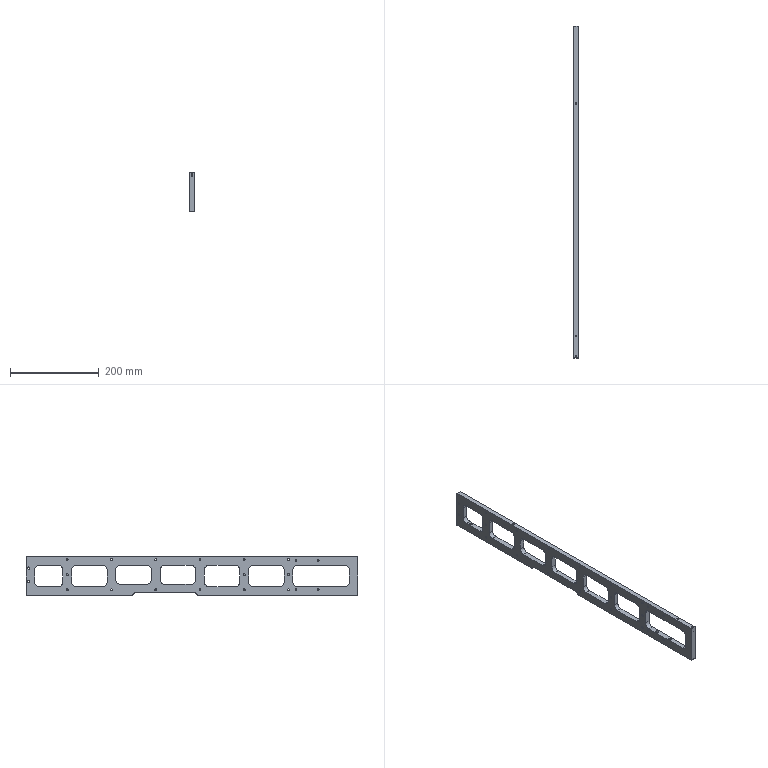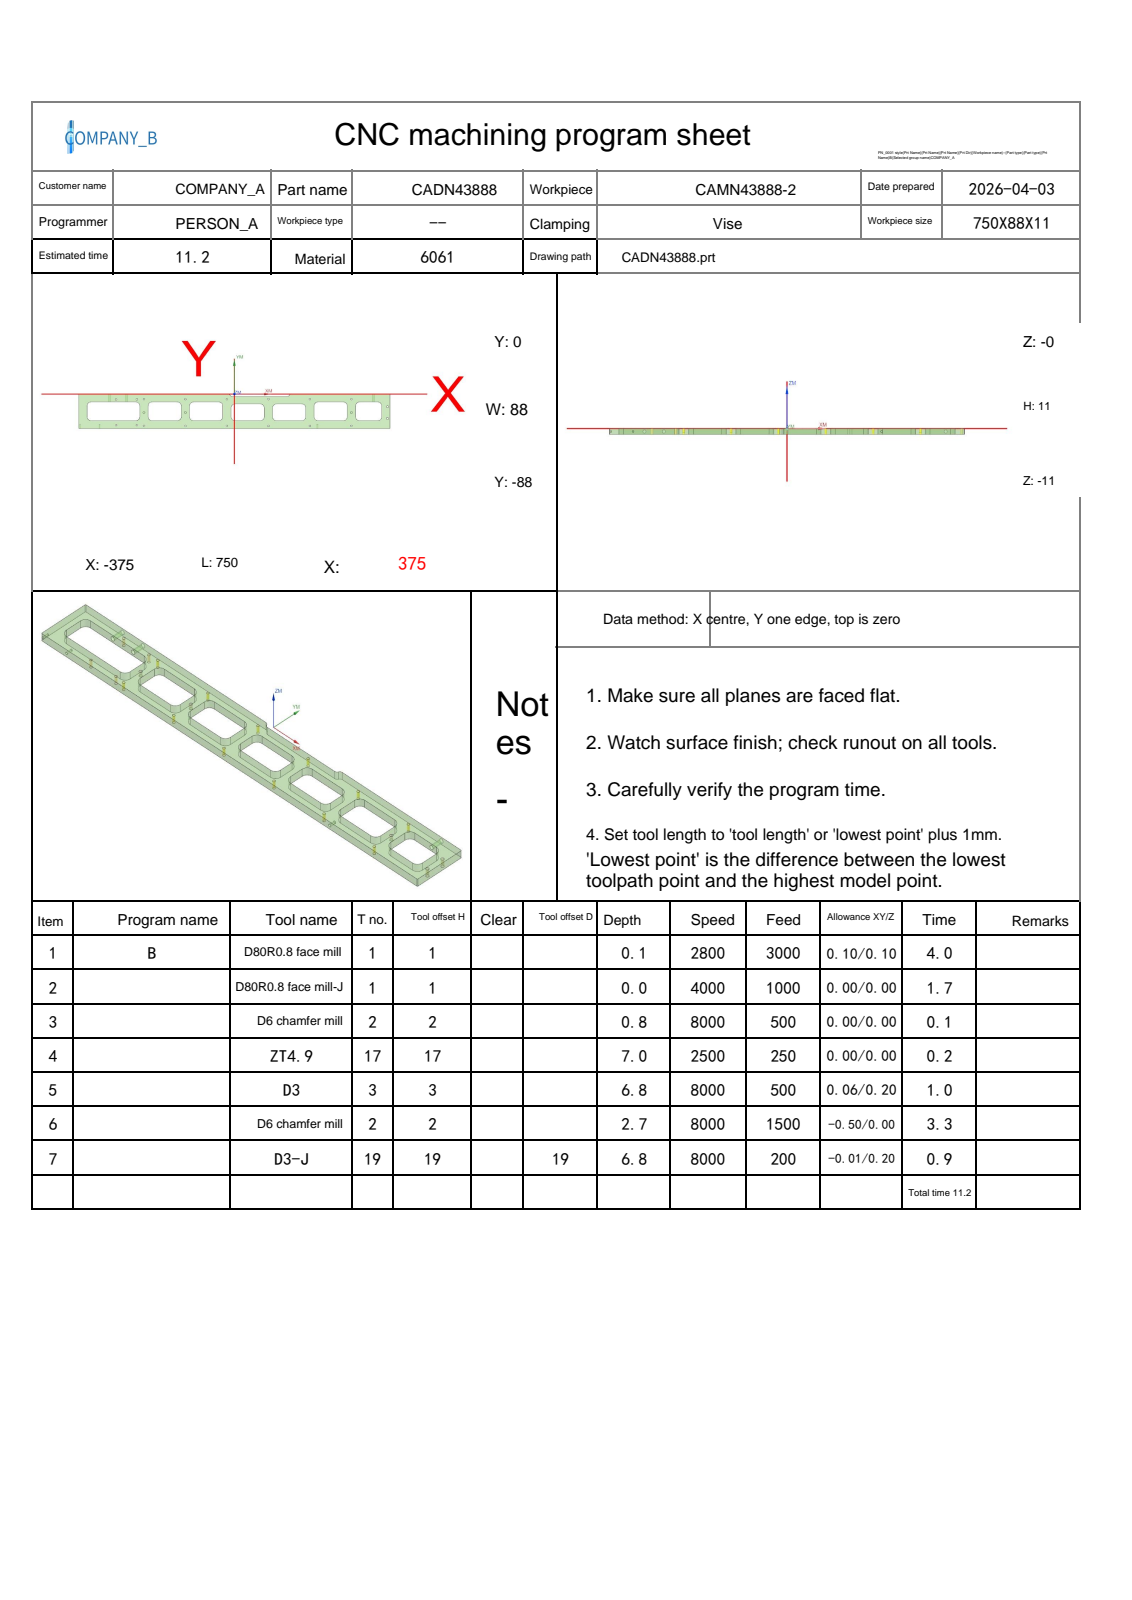NC program | NX | posted by the shop | part box 11 x 750 x 88 mm
Whole program:
%
O0001
(Machine time: 12.66 MIN)
(===Total Tool:5===)
(T1=D80R0.8 face mill D=80.  R=0.8  D-  H01 Z=-0.   )
(T2=D6 chamfer mill   D=6.   R=0.   D-  H02 Z=-2.7  )
(T17=ZT4.9  D=4.9  DR_a=120 D-  H17 Z=-7.   )
(T3=D3      D=3.   R=0.   D-  H03 Z=-6.8  )
(T19=D3-J   D=3.   R=0.   D19 H19 Z=-6.8  )
G80 G90 G17 G49 G40
G91 G28 Z0
M01
N1 T01 M06
(D80R0.8 face mill  D=80. R=0.8 H=01 ce=0.10 di=0.10)
G00 G90 G54 X-427.097 Y-24.494 M03 S2800
G43 H01 Z20.
M08
Z5.014
G01 Z3.014 F3000.
X-415.097 Y-24.361
X407.817 Y-15.229
X407.897
G02 X415.097 Y-22.429 I0.0 J-7.2
G01 Y-48.367
G02 X407.186 Y-56.366 I-8. J0.0
G01 X-415.097 Y-65.491
X-427.097 Y-65.624
Z5.014
G00 Y-24.494
Z4.529
G01 Z2.529
X-415.097 Y-24.361
X407.817 Y-15.229
X407.897
G02 X415.097 Y-22.429 I0.0 J-7.2
G01 Y-48.367
G02 X407.186 Y-56.366 I-8. J0.0
G01 X-415.097 Y-65.491
X-427.097 Y-65.624
Z4.529
G00 Y-24.494
Z4.043
G01 Z2.043
X-415.097 Y-24.361
X407.817 Y-15.229
X407.897
G02 X415.097 Y-22.429 I0.0 J-7.2
G01 Y-48.367
G02 X407.186 Y-56.366 I-8. J0.0
G01 X-415.097 Y-65.491
X-427.097 Y-65.624
Z4.043
G00 Y-24.494
Z3.557
G01 Z1.557
X-415.097 Y-24.361
X407.817 Y-15.229
X407.897
G02 X415.097 Y-22.429 I0.0 J-7.2
G01 Y-48.367
G02 X407.186 Y-56.366 I-8. J0.0
G01 X-415.097 Y-65.491
X-427.097 Y-65.624
Z3.557
G00 Y-24.494
Z3.071
G01 Z1.071
X-415.097 Y-24.361
X407.817 Y-15.229
X407.897
G02 X415.097 Y-22.429 I0.0 J-7.2
G01 Y-48.367
G02 X407.186 Y-56.366 I-8. J0.0
G01 X-415.097 Y-65.491
X-427.097 Y-65.624
Z3.071
G00 Y-24.494
Z2.586
G01 Z.586
X-415.097 Y-24.361
X407.817 Y-15.229
X407.897
G02 X415.097 Y-22.429 I0.0 J-7.2
G01 Y-48.367
G02 X407.186 Y-56.366 I-8. J0.0
G01 X-415.097 Y-65.491
X-427.097 Y-65.624
Z2.586
G00 Y-24.494
Z2.1
G01 Z.1
X-415.097 Y-24.361
X407.817 Y-15.229
X407.897
G02 X415.097 Y-22.429 I0.0 J-7.2
G01 Y-48.367
G02 X407.186 Y-56.366 I-8. J0.0
G01 X-415.097 Y-65.491
X-427.097 Y-65.624
Z2.1
G00 Z20.
G91 G28 Z0.0
M05
M09
G91 G28 Z0.0
M01
N2 T01 M06
(D80R0.8 face mill-J  D=80. R=0.8 H=01 ce=0.00 di=0.00)
G00 G90 G54 X-426.999 Y-24.589 M03 S4000
G43 H01 Z20.
M08
Z2.
G01 Z0.0 F1000.
X-414.999 Y-24.456
X407.719 Y-15.352
X407.799
G02 X414.999 Y-22.552 I0.0 J-7.2
G01 Y-48.271
G02 X407.088 Y-56.271 I-8. J0.0
G01 X-414.999 Y-65.368
X-426.999 Y-65.501
Z2.
G00 Z20.
G91 G28 Z0.0
M05
M09
G91 G28 Z0.0
M01
N3 T02 M06
(D6 chamfer mill  D=6. R=0. H=02 ce=0.00 di=0.00)
G00 G90 G54 X282. Y-47. M03 S8000
G43 H02 Z20.
M08
G98 G81 X282. Y-47. Z-.8 R1. F500.
X-118.
X-218.
G80
G00 Z20.
G91 G28 Z0.0
M05
M09
G91 G28 Z0.0
M01
N4 T17 M06
(ZT4.9 D=4.9 DR_a=120 H=17)
G00 G90 G54 X282. Y-47. M03 S2500
G43 H17 Z20.
M08
G98 G83 X282. Y-47. Z-7. R1. F250. Q2.
X-118.
X-218.
G80
G00 Z20.
G91 G28 Z0.0
M05
M09
G91 G28 Z0.0
M01
N5 T03 M06
(D3  D=3. R=0. H=03 ce=0.06 di=0.20)
G00 G90 G54 X282. Y-47. M03 S8000
G43 H03 Z20.
M08
Z.5
G03 X282.475 Y-47.475 I.475 J0.0 F500.
X282.95 Y-47. I0.0 J.475
X282.95 Y-47. Z.2 I-.95 J0.0
X282.95 Y-47. Z-.1 I-.95 J0.0
X282.95 Y-47. Z-.4 I-.95 J0.0
X282.95 Y-47. Z-.7 I-.95 J0.0
X282.95 Y-47. Z-1. I-.95 J0.0
X282.95 Y-47. Z-1.3 I-.95 J0.0
X282.95 Y-47. Z-1.6 I-.95 J0.0
X282.95 Y-47. Z-1.9 I-.95 J0.0
X282.95 Y-47. Z-2.2 I-.95 J0.0
X282.95 Y-47. Z-2.5 I-.95 J0.0
X282.95 Y-47. Z-2.8 I-.95 J0.0
X282.95 Y-47. Z-3.1 I-.95 J0.0
X282.95 Y-47. Z-3.4 I-.95 J0.0
X282.95 Y-47. Z-3.7 I-.95 J0.0
X282.95 Y-47. Z-4. I-.95 J0.0
X282.95 Y-47. Z-4.3 I-.95 J0.0
X282.95 Y-47. Z-4.6 I-.95 J0.0
X282.95 Y-47. Z-4.9 I-.95 J0.0
X282.95 Y-47. Z-5.2 I-.95 J0.0
X282.95 Y-47. Z-5.5 I-.95 J0.0
X282.95 Y-47. Z-5.8 I-.95 J0.0
X282.95 Y-47. Z-6.1 I-.95 J0.0
X282.95 Y-47. Z-6.4 I-.95 J0.0
X282.95 Y-47. Z-6.7 I-.95 J0.0
X281.525 Y-46.177 Z-6.8 I-.95 J0.0
X281.05 Y-47. I.475 J-.823
X282. Y-47.95 I.95 J0.0
X282.95 Y-47. I0.0 J.95
X282. Y-46.05 I-.95 J0.0
X281.525 Y-46.177 I0.0 J-.95
X281.288 Y-46.589 I.238 J-.411
X281.763 Y-47.064 I.475 J0.0
X282. Y-47. I0.0 J.475
G00 Z20.
X-118.
Z.5
G03 X-117.525 Y-47.475 I.475 J0.0
X-117.05 Y-47. I0.0 J.475
X-117.05 Y-47. Z.2 I-.95 J0.0
X-117.05 Y-47. Z-.1 I-.95 J0.0
X-117.05 Y-47. Z-.4 I-.95 J0.0
X-117.05 Y-47. Z-.7 I-.95 J0.0
X-117.05 Y-47. Z-1. I-.95 J0.0
X-117.05 Y-47. Z-1.3 I-.95 J0.0
X-117.05 Y-47. Z-1.6 I-.95 J0.0
X-117.05 Y-47. Z-1.9 I-.95 J0.0
X-117.05 Y-47. Z-2.2 I-.95 J0.0
X-117.05 Y-47. Z-2.5 I-.95 J0.0
X-117.05 Y-47. Z-2.8 I-.95 J0.0
X-117.05 Y-47. Z-3.1 I-.95 J0.0
X-117.05 Y-47. Z-3.4 I-.95 J0.0
X-117.05 Y-47. Z-3.7 I-.95 J0.0
X-117.05 Y-47. Z-4. I-.95 J0.0
X-117.05 Y-47. Z-4.3 I-.95 J0.0
X-117.05 Y-47. Z-4.6 I-.95 J0.0
X-117.05 Y-47. Z-4.9 I-.95 J0.0
X-117.05 Y-47. Z-5.2 I-.95 J0.0
X-117.05 Y-47. Z-5.5 I-.95 J0.0
X-117.05 Y-47. Z-5.8 I-.95 J0.0
X-117.05 Y-47. Z-6.1 I-.95 J0.0
X-117.05 Y-47. Z-6.4 I-.95 J0.0
X-117.05 Y-47. Z-6.7 I-.95 J0.0
X-118.475 Y-46.177 Z-6.8 I-.95 J0.0
X-118.95 Y-47. I.475 J-.823
X-118. Y-47.95 I.95 J0.0
X-117.05 Y-47. I0.0 J.95
X-118. Y-46.05 I-.95 J0.0
X-118.475 Y-46.177 I0.0 J-.95
X-118.712 Y-46.589 I.238 J-.411
X-118.237 Y-47.064 I.475 J0.0
X-118. Y-47. I0.0 J.475
G00 Z20.
X-218.
Z.5
G03 X-217.525 Y-47.475 I.475 J0.0
X-217.05 Y-47. I0.0 J.475
X-217.05 Y-47. Z.2 I-.95 J0.0
X-217.05 Y-47. Z-.1 I-.95 J0.0
X-217.05 Y-47. Z-.4 I-.95 J0.0
X-217.05 Y-47. Z-.7 I-.95 J0.0
X-217.05 Y-47. Z-1. I-.95 J0.0
X-217.05 Y-47. Z-1.3 I-.95 J0.0
X-217.05 Y-47. Z-1.6 I-.95 J0.0
X-217.05 Y-47. Z-1.9 I-.95 J0.0
X-217.05 Y-47. Z-2.2 I-.95 J0.0
X-217.05 Y-47. Z-2.5 I-.95 J0.0
X-217.05 Y-47. Z-2.8 I-.95 J0.0
X-217.05 Y-47. Z-3.1 I-.95 J0.0
X-217.05 Y-47. Z-3.4 I-.95 J0.0
X-217.05 Y-47. Z-3.7 I-.95 J0.0
X-217.05 Y-47. Z-4. I-.95 J0.0
X-217.05 Y-47. Z-4.3 I-.95 J0.0
X-217.05 Y-47. Z-4.6 I-.95 J0.0
X-217.05 Y-47. Z-4.9 I-.95 J0.0
X-217.05 Y-47. Z-5.2 I-.95 J0.0
X-217.05 Y-47. Z-5.5 I-.95 J0.0
X-217.05 Y-47. Z-5.8 I-.95 J0.0
X-217.05 Y-47. Z-6.1 I-.95 J0.0
X-217.05 Y-47. Z-6.4 I-.95 J0.0
X-217.05 Y-47. Z-6.7 I-.95 J0.0
X-218.475 Y-46.177 Z-6.8 I-.95 J0.0
X-218.95 Y-47. I.475 J-.823
X-218. Y-47.95 I.95 J0.0
X-217.05 Y-47. I0.0 J.95
X-218. Y-46.05 I-.95 J0.0
X-218.475 Y-46.177 I0.0 J-.95
X-218.712 Y-46.589 I.238 J-.411
X-218.237 Y-47.064 I.475 J0.0
X-218. Y-47. I0.0 J.475
G00 Z20.
G91 G28 Z0.0
M05
M09
G91 G28 Z0.0
M01
N6 T02 M06
(D6 chamfer mill  D=6. R=0. H=02 ce=0.00 di=0.20)
G00 G90 G54 X-218. Y-81. M03 S5000
G43 H02 Z20.
M08
G98 G81 X-218. Y-81. Z-2.7 R3. F150.
X-235. Y-79.25
X-285.
Y-13.75
X-235.
X-218. Y-13.
X-118.
Y-81.
X-18.
Y-13.
X82.
Y-81.
X182.
Y-13.
X282.
Y-81.
G80
G00 Z20.
G00 G90 X-217.044 Y-46.675 M03 S8000
Z20.
Z-.5
G01 Z-1. F500.
X-216.5 Y-46.49
G03 X-218. Y-44.99 I-1.5 J0.0
X-220.01 Y-47. I0.0 J-2.01
X-218. Y-49.01 I2.01 J0.0
X-215.99 Y-47. I0.0 J2.01
X-218. Y-44.99 I-2.01 J0.0
X-219.5 Y-46.49 I0.0 J-1.5
G01 X-218.956 Y-46.675
Z-.5
G00 Z20.
X-117.044
Z-.5
G01 Z-1.
X-116.5 Y-46.49
G03 X-118. Y-44.99 I-1.5 J0.0
X-120.01 Y-47. I0.0 J-2.01
X-118. Y-49.01 I2.01 J0.0
X-115.99 Y-47. I0.0 J2.01
X-118. Y-44.99 I-2.01 J0.0
X-119.5 Y-46.49 I0.0 J-1.5
G01 X-118.956 Y-46.675
Z-.5
G00 Z20.
X282.956
Z-.5
G01 Z-1.
X283.5 Y-46.49
G03 X282. Y-44.99 I-1.5 J0.0
X279.99 Y-47. I0.0 J-2.01
X282. Y-49.01 I2.01 J0.0
X284.01 Y-47. I0.0 J2.01
X282. Y-44.99 I-2.01 J0.0
X280.5 Y-46.49 I0.0 J-1.5
G01 X281.044 Y-46.675
Z-.5
G00 Z20.
G00 G90 X-354. Y-47.01 M03 S7000
Z20.
Z2.5
G01 Y-58. Z-1.5 F1500.
G03 X-345. Y-67. I9. J0.0
G01 X-238.
G03 X-229. Y-58. I0.0 J9.
G01 Y-30.
G03 X-238. Y-21. I-9. J0.0
G01 X-345.
G03 X-354. Y-30. I0.0 J-9.
G01 Y-58.
G03 X-353.986 Y-58.5 I9. J0.0
G01 Z1.
G00 Z20.
X-207. Y-47.01
Z2.5
G01 Y-58. Z-1.5
G03 X-198. Y-67. I9. J0.0
G01 X-138.
G03 X-129. Y-58. I0.0 J9.
G01 Y-30.
G03 X-138. Y-21. I-9. J0.0
G01 X-198.
G03 X-207. Y-30. I0.0 J-9.
G01 Y-58.
G03 X-206.986 Y-58.5 I9. J0.0
G01 Z1.
G00 Z20.
X-107. Y-47.01
Z2.5
G01 Y-58. Z-1.5
G03 X-98. Y-67. I9. J0.0
G01 X-38.
G03 X-29. Y-58. I0.0 J9.
G01 Y-30.
G03 X-38. Y-21. I-9. J0.0
G01 X-98.
G03 X-107. Y-30. I0.0 J-9.
G01 Y-58.
G03 X-106.986 Y-58.5 I9. J0.0
G01 Z1.
G00 Z20.
X117.01 Y-5.
Z2.5
G01 X128. Z-1.5
G03 X131.666 Y-2.6 I0.0 J4.
G02 X137.165 Y1. I5.499 J-2.4
G01 X374.
G02 X376. Y-1. I0.0 J-2.
G01 Y-87.
G02 X374. Y-89. I-2. J0.0
G01 X-374.
G02 X-376. Y-87. I0.0 J2.
G01 Y-1.
G02 X-374. Y1. I2. J0.0
G01 X-15.165
G02 X-9.666 Y-2.6 I0.0 J-6.
G03 X-6. Y-5. I3.666 J1.6
G01 X128.
G03 X128.499 Y-4.969 I0.0 J4.
G01 Z1.
G00 Z20.
X-7. Y-47.01
Z2.5
G01 Y-58. Z-1.5
G03 X2. Y-67. I9. J0.0
G01 X62.
G03 X71. Y-58. I0.0 J9.
G01 Y-35.
G03 X62. Y-26. I-9. J0.0
G01 X2.
G03 X-7. Y-35. I0.0 J-9.
G01 Y-58.
G03 X-6.986 Y-58.5 I9. J0.0
G01 Z1.
G00 Z20.
X93. Y-47.01
Z2.5
G01 Y-58. Z-1.5
G03 X102. Y-67. I9. J0.0
G01 X162.
G03 X171. Y-58. I0.0 J9.
G01 Y-35.
G03 X162. Y-26. I-9. J0.0
G01 X102.
G03 X93. Y-35. I0.0 J-9.
G01 Y-58.
G03 X93.014 Y-58.5 I9. J0.0
G01 Z1.
G00 Z20.
X193. Y-47.01
Z2.5
G01 Y-58. Z-1.5
G03 X202. Y-67. I9. J0.0
G01 X262.
G03 X271. Y-58. I0.0 J9.
G01 Y-30.
G03 X262. Y-21. I-9. J0.0
G01 X202.
G03 X193. Y-30. I0.0 J-9.
G01 Y-58.
G03 X193.014 Y-58.5 I9. J0.0
G01 Z1.
G00 Z20.
X293. Y-47.01
Z2.5
G01 Y-58. Z-1.5
G03 X302. Y-67. I9. J0.0
G01 X345.
G03 X354. Y-58. I0.0 J9.
G01 Y-30.
G03 X345. Y-21. I-9. J0.0
G01 X302.
G03 X293. Y-30. I0.0 J-9.
G01 Y-58.
G03 X293.014 Y-58.5 I9. J0.0
G01 Z1.
G00 Z20.
G91 G28 Z0.0
M05
M09
G91 G28 Z0.0
M01
N7 T19 M06
(D3-J  D=3. R=0. H=19 ce=-0.01 di=0.20)
G00 G90 G54 X282. Y-47. M03 S8000
G43 H19 Z20.
M08
Z.5
G41 D19
G01 X282.076 Y-47.185 F200.
G03 X282.53 Y-47.49 I.454 J.185
X283.02 Y-47. I0.0 J.49
X283.02 Y-47. Z-.5 I-1.02 J0.0
X283.02 Y-47. Z-1.5 I-1.02 J0.0
X283.02 Y-47. Z-2.5 I-1.02 J0.0
X283.02 Y-47. Z-3.5 I-1.02 J0.0
X283.02 Y-47. Z-4.5 I-1.02 J0.0
X283.02 Y-47. Z-5.5 I-1.02 J0.0
X283.02 Y-47. Z-6.5 I-1.02 J0.0
X281.685 Y-46.03 Z-6.8 I-1.02 J0.0
X280.98 Y-47. I.315 J-.97
X282. Y-48.02 I1.02 J0.0
X283.02 Y-47. I0.0 J1.02
X282. Y-45.98 I-1.02 J0.0
X281.685 Y-46.03 I0.0 J-1.02
X281.346 Y-46.496 I.152 J-.466
X281.801 Y-46.985 I.49 J0.0
G01 G40 X282. Y-47.
G00 Z20.
X-118.
Z.5
G41 D19
G01 X-117.924 Y-47.185
G03 X-117.47 Y-47.49 I.454 J.185
X-116.98 Y-47. I0.0 J.49
X-116.98 Y-47. Z-.5 I-1.02 J0.0
X-116.98 Y-47. Z-1.5 I-1.02 J0.0
X-116.98 Y-47. Z-2.5 I-1.02 J0.0
X-116.98 Y-47. Z-3.5 I-1.02 J0.0
X-116.98 Y-47. Z-4.5 I-1.02 J0.0
X-116.98 Y-47. Z-5.5 I-1.02 J0.0
X-116.98 Y-47. Z-6.5 I-1.02 J0.0
X-118.315 Y-46.03 Z-6.8 I-1.02 J0.0
X-119.02 Y-47. I.315 J-.97
X-118. Y-48.02 I1.02 J0.0
X-116.98 Y-47. I0.0 J1.02
X-118. Y-45.98 I-1.02 J0.0
X-118.315 Y-46.03 I0.0 J-1.02
X-118.654 Y-46.496 I.152 J-.466
X-118.199 Y-46.985 I.49 J0.0
G01 G40 X-118. Y-47.
G00 Z20.
X-218.
Z.5
G41 D19
G01 X-217.924 Y-47.185
G03 X-217.47 Y-47.49 I.454 J.185
X-216.98 Y-47. I0.0 J.49
X-216.98 Y-47. Z-.5 I-1.02 J0.0
X-216.98 Y-47. Z-1.5 I-1.02 J0.0
X-216.98 Y-47. Z-2.5 I-1.02 J0.0
X-216.98 Y-47. Z-3.5 I-1.02 J0.0
X-216.98 Y-47. Z-4.5 I-1.02 J0.0
X-216.98 Y-47. Z-5.5 I-1.02 J0.0
X-216.98 Y-47. Z-6.5 I-1.02 J0.0
X-218.315 Y-46.03 Z-6.8 I-1.02 J0.0
X-219.02 Y-47. I.315 J-.97
X-218. Y-48.02 I1.02 J0.0
X-216.98 Y-47. I0.0 J1.02
X-218. Y-45.98 I-1.02 J0.0
X-218.315 Y-46.03 I0.0 J-1.02
X-218.654 Y-46.496 I.152 J-.466
X-218.199 Y-46.985 I.49 J0.0
G01 G40 X-218. Y-47.
G00 Z20.
M05
M09
G91 G28 Z0.0
G91 G28 Y0.0
M30
%